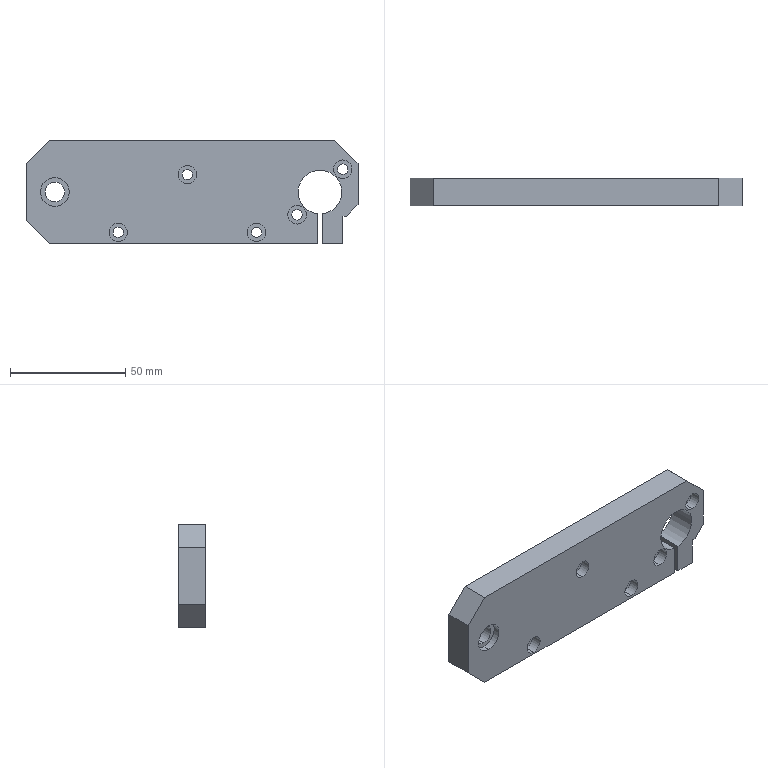Part | STEP file | PN_0046 | 1 solid | 60 faces | box 144 x 12 x 45 mm | volume 67965 mm3 | cylinder 33 | plane 21 | cone 6 | commonest cylinder face diameters 4.5 x10 8 x10 3 x4 4.2 x2 5.5 x2 8.5 x2